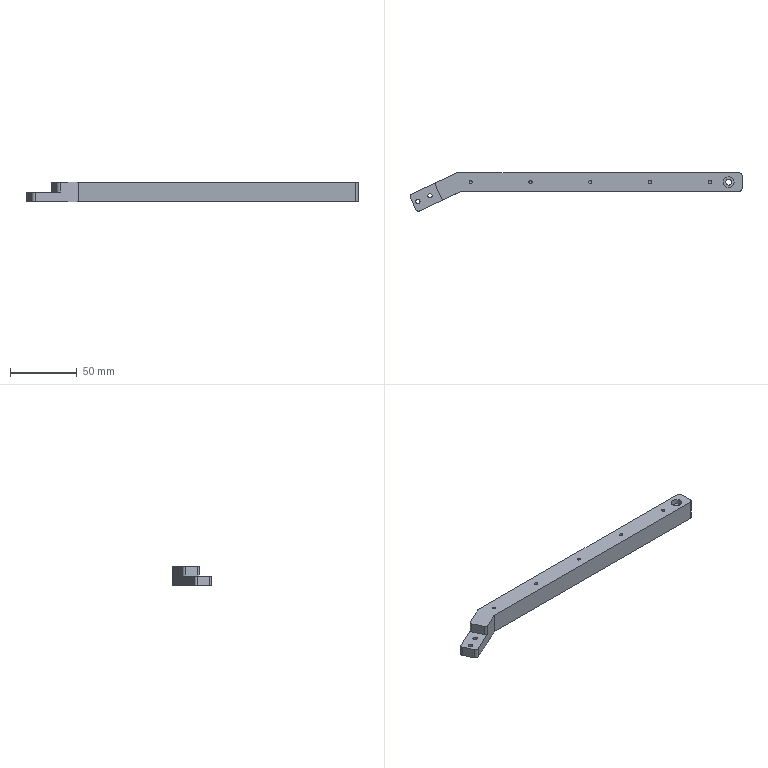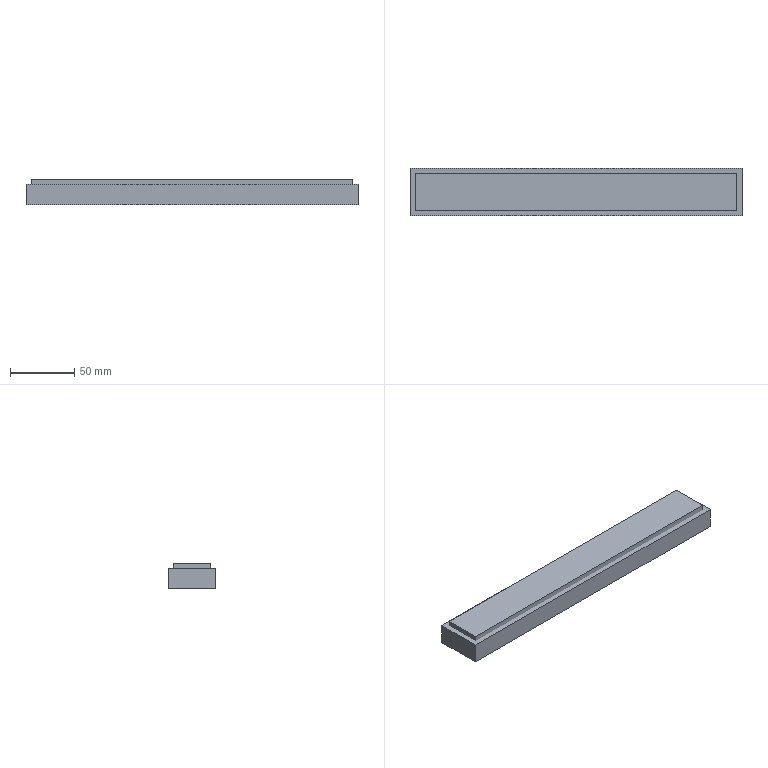CAM job | NX | 3-axis milling, drilling | part box 249.594 x 28.935 x 15 mm | stock box 257.594 x 36.935 x 20 mm
Tools:
number,name,description,diameter,corner_radius,flute_length,length,flutes
1,D63,Milling Tool-5 Parameters,63.0,0.0,50.0,75.0,2
2,D10,Milling Tool-5 Parameters,10.0,0.0,50.0,75.0,2
9,D6A45,Milling Tool-5 Parameters,6.0,0.0,3.0,3.0,2
16,4.2ZT,Drilling Tool,3.2,0.0,35.0,50.0,2
10,2.5ZT,Drilling Tool,2.4,0.0,35.0,50.0,2
14,4.5ZT,Drilling Tool,4.5,0.0,35.0,50.0,2
4,D6,Milling Tool-5 Parameters,6.0,0.0,50.0,75.0,2
Operations:
program,operation,operation_type,tool,method,geometry_group,spindle_rpm,surface_speed,feed_per_tooth,feed_cut,feed_plunge,cut_length_mm,path_length_mm,cut_time_min,machine_time_min
1-255-35-20毛胚,FLOOR_WALL,VolumeBased25DMillingOperation,D63,METHOD,A,6500.0,0.0,0.0,1250.0,100.0,332.594,386.594,0.2661,0.2715
1-255-35-20毛胚,ADAPTIVE_MILLING,CavityMilling,D10,METHOD,A,7000.0,219.0,0.1429,2000.0,1000.0,9397.311,15455.481,4.73,5.336
1-255-35-20毛胚,ZLEVEL_PROFILE_COPY_COPY_1_COPY,ZLevelMilling,D10,METHOD,A,6500.0,326.0,0.0769,1000.0,1000.0,566.789,653.789,0.5668,0.5755
1-255-35-20毛胚,FLOOR_WALL_1_COPY_COPY_1_COPY,VolumeBased25DMillingOperation,D10,METHOD,A,7000.0,219.0,0.0714,1000.0,1000.0,153.952,330.6,0.154,0.1716
1-255-35-20毛胚,DRILLING,Operation,D6A45,METHOD,A,4000.0,75.0,0.0312,250.0,0.0,32.0,390.272,0.128,0.1638
1-255-35-20毛胚,DRILLING_COPY_1,Operation,4.2ZT,METHOD,A,2000.0,20.0,0.05,200.0,0.0,25.923,140.286,0.1296,0.1411
1-255-35-20毛胚,DRILLING_COPY_1_COPY,Operation,2.5ZT,METHOD,A,2000.0,20.0,0.05,120.0,0.0,58.549,369.498,0.4879,0.519
1-255-35-20毛胚,DRILLING_COPY_1_COPY_1,Operation,4.5ZT,METHOD,A,2000.0,20.0,0.05,200.0,0.0,20.852,101.704,0.1043,0.1123
1-255-35-20毛胚,HOLE_MILLING,CylinderMilling,D6,METHOD,A,7000.0,131.0,0.1214,1700.0,100.0,80.254,143.754,0.0472,0.0536
1-255-35-20毛胚,ZLEVEL_PROFILE_COPY_1_COPY_COPY_COPY_COPY,ZLevelMilling,D6A45,METHOD,A,7000.0,131.0,0.0714,1000.0,1000.0,533.819,1495.813,0.5338,0.63
1-255-35-20毛胚,ZLEVEL_PROFILE_COPY_1_COPY_COPY_COPY_COPY_COPY,ZLevelMilling,D6A45,METHOD,A,7000.0,131.0,0.0714,1000.0,1000.0,67.471,316.346,0.0675,0.0924
2-255-35-20毛胚,FLOOR_WALL_COPY,VolumeBased25DMillingOperation,D63,METHOD,B,6500.0,0.0,0.0,1250.0,100.0,1622.972,3147.351,1.298,1.451
2-255-35-20毛胚,ZLEVEL_PROFILE_COPY_1_COPY_COPY_COPY_COPY_COPY_COPY,ZLevelMilling,D6A45,METHOD,B,7000.0,131.0,0.0714,1000.0,1000.0,559.073,1062.103,0.5591,0.6094